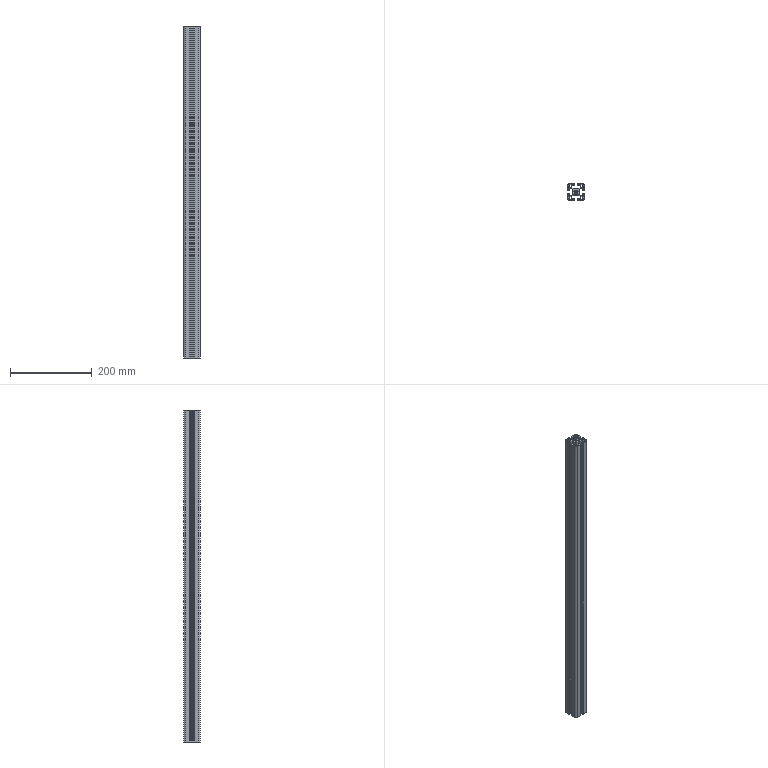Part | SolidWorks | features HoleWzd 2, Extrusion 1 | 1 solid | 182 faces | box 40 x 40 x 810 mm | volume 486492 mm3 | plane 137 | cylinder 45 | commonest cylinder face diameters 1 x8 2 x8 6.6 x8 6.8 x8 5 x4 9 x4